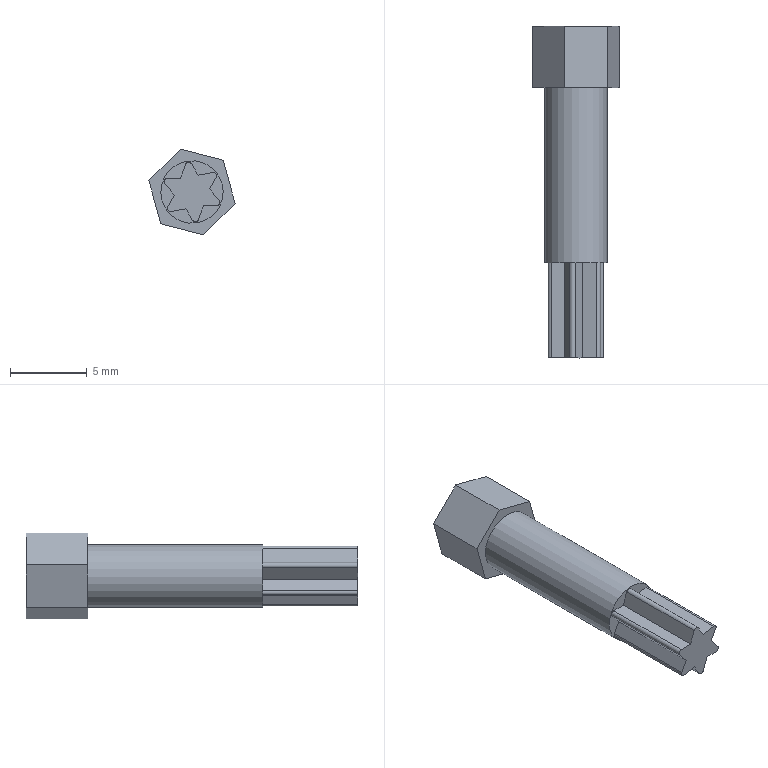Part | STEP file | Zapas-_150-001-1 | 1 solid | 31 faces | box 5.61 x 21.6 x 5.588 mm | volume 281.637 mm3 | plane 22 | cylinder 9 | commonest cylinder face diameters 0.42 x8 4.06 x1